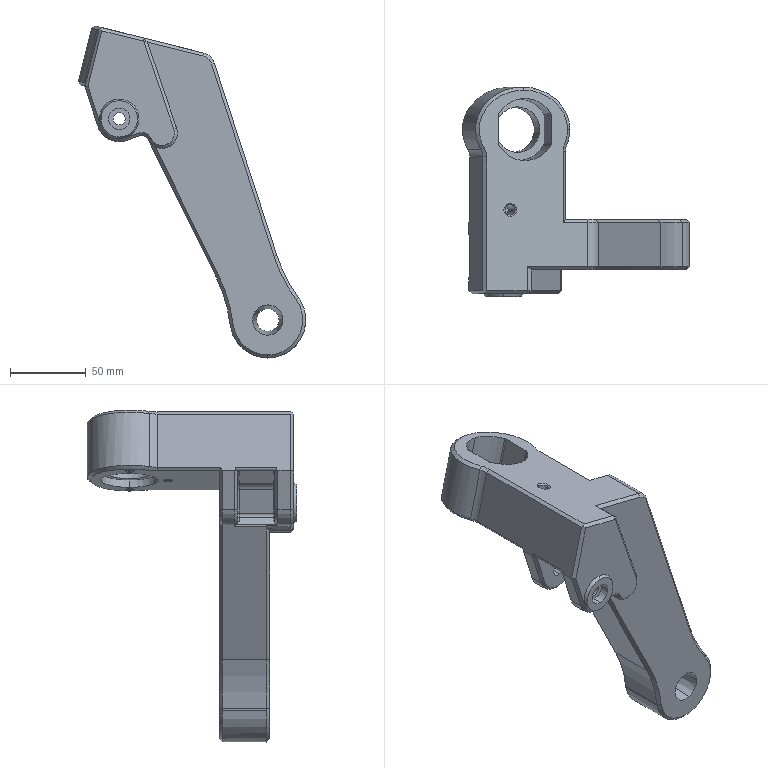Part | SolidWorks | features BaseBody 1 | 1 solid | 180 faces | box 149.695 x 138 x 218.474 mm | volume 579562 mm3 | cylinder 58 | plane 57 | cone 50 | spline 11 | torus 4 | commonest cylinder face diameters 2 x7 30 x7 4.8 x6 20 x6 4.116 x4 7.95 x4